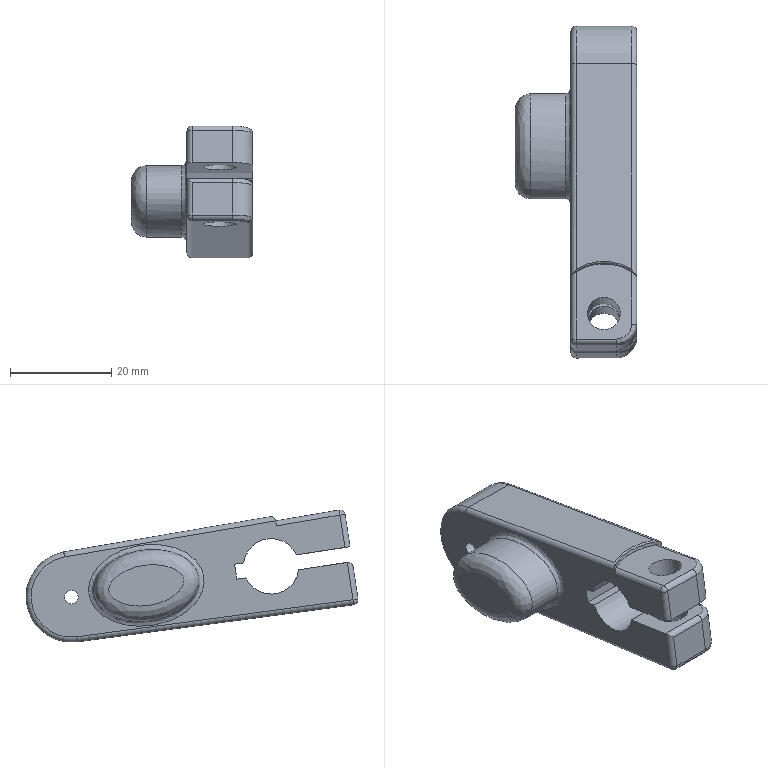Part | NX | features BREP 1 | 1 solid | 48 faces | box 24 x 65.725 x 26.174 mm | volume 14639 mm3 | cylinder 22 | plane 13 | spline 5 | torus 4 | cone 2 | sphere 2 | commonest cylinder face diameters 2 x12 6 x2 6.5 x2 8 x2 11 x2 18 x1